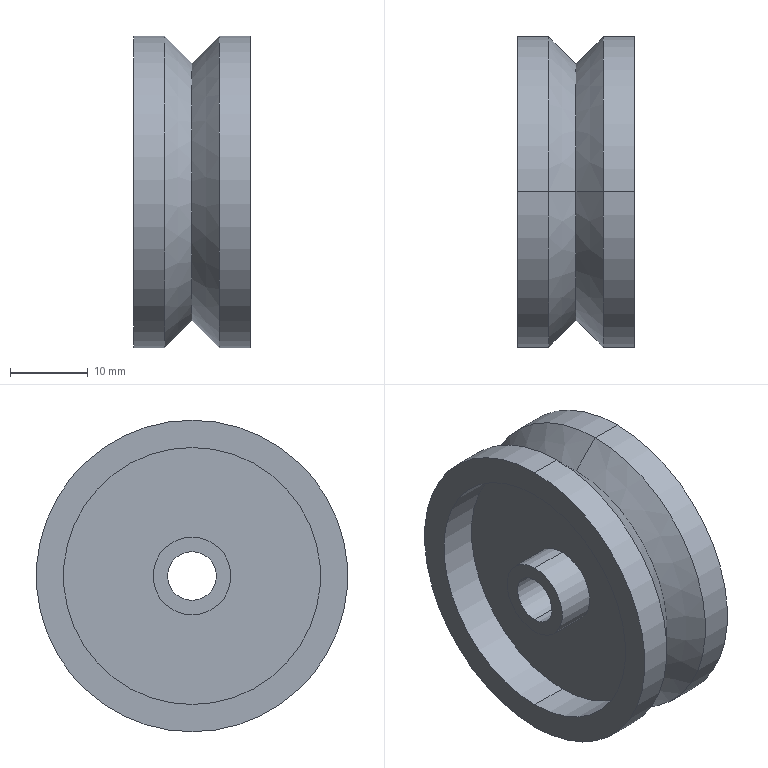Part | SolidWorks | features Revolution 1 | 1 solid | 24 faces | box 15 x 40 x 40 mm | volume 9172 mm3 | cylinder 14 | plane 6 | cone 4 | commonest cylinder face diameters 10 x4 33 x4 40 x4 6.25 x2
STEP:
#1=CARTESIAN_POINT('',(0.,0.,0.6496));
#2=VERTEX_POINT('',#1);
#3=CARTESIAN_POINT('',(0.,0.,-0.6496));
#4=VERTEX_POINT('',#3);
#5=CARTESIAN_POINT('',(0.,0.,0.));
#6=DIRECTION('',(-1.,0.,0.));
#7=DIRECTION('',(0.,0.,1.));
#8=AXIS2_PLACEMENT_3D('',#5,#6,#7);
#9=CIRCLE('',#8,0.6496);
#10=EDGE_CURVE('',#2,#4,#9,.T.);
#11=ORIENTED_EDGE('',*,*,#10,.F.);
#12=CARTESIAN_POINT('',(0.1378,0.,0.7874));
#13=VERTEX_POINT('',#12);
#14=CARTESIAN_POINT('',(0.1378,0.,0.7874));
#15=DIRECTION('',(0.7071,0.,0.7071));
#16=VECTOR('',#15,39.37);
#17=LINE('',#14,#16);
#18=EDGE_CURVE('',#2,#13,#17,.T.);
#19=ORIENTED_EDGE('',*,*,#18,.T.);
#20=CARTESIAN_POINT('',(0.1378,0.,-0.7874));
#21=VERTEX_POINT('',#20);
#22=CARTESIAN_POINT('',(0.1378,0.,0.));
#23=DIRECTION('',(-1.,0.,0.));
#24=DIRECTION('',(0.,0.,1.));
#25=AXIS2_PLACEMENT_3D('',#22,#23,#24);
#26=CIRCLE('',#25,0.7874);
#27=EDGE_CURVE('',#13,#21,#26,.T.);
#28=ORIENTED_EDGE('',*,*,#27,.T.);
#29=CARTESIAN_POINT('',(0.1378,0.,-0.7874));
#30=DIRECTION('',(0.7071,0.,-0.7071));
#31=VECTOR('',#30,39.37);
#32=LINE('',#29,#31);
#33=EDGE_CURVE('',#4,#21,#32,.T.);
#34=ORIENTED_EDGE('',*,*,#33,.F.);
#35=EDGE_LOOP('',(#11,#19,#28,#34));
#36=FACE_OUTER_BOUND('',#35,.T.);
#37=CARTESIAN_POINT('',(0.1378,0.,0.));
#38=DIRECTION('',(1.,0.,0.));
#39=DIRECTION('',(0.,0.,-1.));
#40=AXIS2_PLACEMENT_3D('',#37,#38,#39);
#41=CONICAL_SURFACE('',#40,0.7874,0.7854);
#42=ADVANCED_FACE('',(#36),#41,.T.);
#43=CARTESIAN_POINT('',(0.2953,0.,0.7874));
#44=VERTEX_POINT('',#43);
#45=CARTESIAN_POINT('',(0.2953,0.,-0.7874));
#46=VERTEX_POINT('',#45);
#47=CARTESIAN_POINT('',(0.2953,0.,0.));
#48=DIRECTION('',(-1.,0.,0.));
#49=DIRECTION('',(0.,0.,1.));
#50=AXIS2_PLACEMENT_3D('',#47,#48,#49);
#51=CIRCLE('',#50,0.7874);
#52=EDGE_CURVE('',#44,#46,#51,.T.);
#53=ORIENTED_EDGE('',*,*,#52,.T.);
#54=CARTESIAN_POINT('',(-1.791,0.,-0.7874));
#55=DIRECTION('',(-1.,0.,0.));
#56=VECTOR('',#55,39.37);
#57=LINE('',#54,#56);
#58=EDGE_CURVE('',#46,#21,#57,.T.);
#59=ORIENTED_EDGE('',*,*,#58,.T.);
#60=ORIENTED_EDGE('',*,*,#27,.F.);
#61=CARTESIAN_POINT('',(-1.791,0.,0.7874));
#62=DIRECTION('',(-1.,0.,0.));
#63=VECTOR('',#62,39.37);
#64=LINE('',#61,#63);
#65=EDGE_CURVE('',#44,#13,#64,.T.);
#66=ORIENTED_EDGE('',*,*,#65,.F.);
#67=EDGE_LOOP('',(#53,#59,#60,#66));
#68=FACE_OUTER_BOUND('',#67,.T.);
#69=CARTESIAN_POINT('',(-1.791,0.,0.));
#70=DIRECTION('',(-1.,0.,0.));
#71=DIRECTION('',(0.,0.,1.));
#72=AXIS2_PLACEMENT_3D('',#69,#70,#71);
#73=CYLINDRICAL_SURFACE('',#72,0.7874);
#74=ADVANCED_FACE('',(#68),#73,.T.);
#75=CARTESIAN_POINT('',(0.2953,0.,-0.6496));
#76=VERTEX_POINT('',#75);
#77=CARTESIAN_POINT('',(0.2953,0.,0.6496));
#78=VERTEX_POINT('',#77);
#79=CARTESIAN_POINT('',(0.2953,0.,0.));
#80=DIRECTION('',(-1.,0.,0.));
#81=DIRECTION('',(0.,0.,1.));
#82=AXIS2_PLACEMENT_3D('',#79,#80,#81);
#83=CIRCLE('',#82,0.6496);
#84=EDGE_CURVE('',#76,#78,#83,.T.);
#85=ORIENTED_EDGE('',*,*,#84,.F.);
#86=CARTESIAN_POINT('',(0.09843,0.,-0.6496));
#87=VERTEX_POINT('',#86);
#88=CARTESIAN_POINT('',(-1.791,0.,-0.6496));
#89=DIRECTION('',(-1.,0.,0.));
#90=VECTOR('',#89,39.37);
#91=LINE('',#88,#90);
#92=EDGE_CURVE('',#76,#87,#91,.T.);
#93=ORIENTED_EDGE('',*,*,#92,.T.);
#94=CARTESIAN_POINT('',(0.09843,0.,0.6496));
#95=VERTEX_POINT('',#94);
#96=CARTESIAN_POINT('',(0.09843,0.,0.));
#97=DIRECTION('',(-1.,0.,0.));
#98=DIRECTION('',(0.,0.,1.));
#99=AXIS2_PLACEMENT_3D('',#96,#97,#98);
#100=CIRCLE('',#99,0.6496);
#101=EDGE_CURVE('',#87,#95,#100,.T.);
#102=ORIENTED_EDGE('',*,*,#101,.T.);
#103=CARTESIAN_POINT('',(-1.791,0.,0.6496));
#104=DIRECTION('',(-1.,0.,0.));
#105=VECTOR('',#104,39.37);
#106=LINE('',#103,#105);
#107=EDGE_CURVE('',#78,#95,#106,.T.);
#108=ORIENTED_EDGE('',*,*,#107,.F.);
#109=EDGE_LOOP('',(#85,#93,#102,#108));
#110=FACE_OUTER_BOUND('',#109,.T.);
#111=CARTESIAN_POINT('',(-1.791,0.,0.));
#112=DIRECTION('',(-1.,0.,0.));
#113=DIRECTION('',(0.,0.,1.));
#114=AXIS2_PLACEMENT_3D('',#111,#112,#113);
#115=CYLINDRICAL_SURFACE('',#114,0.6496);
#116=ADVANCED_FACE('',(#110),#115,.F.);
#117=CARTESIAN_POINT('',(0.2953,0.,0.1969));
#118=VERTEX_POINT('',#117);
#119=CARTESIAN_POINT('',(0.2953,0.,-0.1969));
#120=VERTEX_POINT('',#119);
#121=CARTESIAN_POINT('',(0.2953,0.,0.));
#122=DIRECTION('',(-1.,0.,0.));
#123=DIRECTION('',(0.,0.,1.));
#124=AXIS2_PLACEMENT_3D('',#121,#122,#123);
#125=CIRCLE('',#124,0.1969);
#126=EDGE_CURVE('',#118,#120,#125,.T.);
#127=ORIENTED_EDGE('',*,*,#126,.T.);
#128=CARTESIAN_POINT('',(0.09843,0.,-0.1969));
#129=VERTEX_POINT('',#128);
#130=CARTESIAN_POINT('',(-1.791,0.,-0.1969));
#131=DIRECTION('',(-1.,0.,0.));
#132=VECTOR('',#131,39.37);
#133=LINE('',#130,#132);
#134=EDGE_CURVE('',#120,#129,#133,.T.);
#135=ORIENTED_EDGE('',*,*,#134,.T.);
#136=CARTESIAN_POINT('',(0.09843,0.,0.1969));
#137=VERTEX_POINT('',#136);
#138=CARTESIAN_POINT('',(0.09843,0.,0.));
#139=DIRECTION('',(-1.,0.,0.));
#140=DIRECTION('',(0.,0.,1.));
#141=AXIS2_PLACEMENT_3D('',#138,#139,#140);
#142=CIRCLE('',#141,0.1969);
#143=EDGE_CURVE('',#137,#129,#142,.T.);
#144=ORIENTED_EDGE('',*,*,#143,.F.);
#145=CARTESIAN_POINT('',(-1.791,0.,0.1969));
#146=DIRECTION('',(-1.,0.,0.));
#147=VECTOR('',#146,39.37);
#148=LINE('',#145,#147);
#149=EDGE_CURVE('',#118,#137,#148,.T.);
#150=ORIENTED_EDGE('',*,*,#149,.F.);
#151=EDGE_LOOP('',(#127,#135,#144,#150));
#152=FACE_OUTER_BOUND('',#151,.T.);
#153=CARTESIAN_POINT('',(-1.791,0.,0.));
#154=DIRECTION('',(-1.,0.,0.));
#155=DIRECTION('',(0.,0.,1.));
#156=AXIS2_PLACEMENT_3D('',#153,#154,#155);
#157=CYLINDRICAL_SURFACE('',#156,0.1969);
#158=ADVANCED_FACE('',(#152),#157,.T.);
#159=CARTESIAN_POINT('',(0.2953,0.,-0.123));
#160=VERTEX_POINT('',#159);
#161=CARTESIAN_POINT('',(0.2953,0.,0.123));
#162=VERTEX_POINT('',#161);
#163=CARTESIAN_POINT('',(0.2953,0.,0.));
#164=DIRECTION('',(-1.,0.,0.));
#165=DIRECTION('',(0.,0.,1.));
#166=AXIS2_PLACEMENT_3D('',#163,#164,#165);
#167=CIRCLE('',#166,0.123);
#168=EDGE_CURVE('',#160,#162,#167,.T.);
#169=ORIENTED_EDGE('',*,*,#168,.F.);
#170=CARTESIAN_POINT('',(-0.2953,0.,-0.123));
#171=VERTEX_POINT('',#170);
#172=CARTESIAN_POINT('',(-1.791,0.,-0.123));
#173=DIRECTION('',(-1.,0.,0.));
#174=VECTOR('',#173,39.37);
#175=LINE('',#172,#174);
#176=EDGE_CURVE('',#160,#171,#175,.T.);
#177=ORIENTED_EDGE('',*,*,#176,.T.);
#178=CARTESIAN_POINT('',(-0.2953,0.,0.123));
#179=VERTEX_POINT('',#178);
#180=CARTESIAN_POINT('',(-0.2953,0.,0.));
#181=DIRECTION('',(-1.,0.,0.));
#182=DIRECTION('',(0.,0.,1.));
#183=AXIS2_PLACEMENT_3D('',#180,#181,#182);
#184=CIRCLE('',#183,0.123);
#185=EDGE_CURVE('',#171,#179,#184,.T.);
#186=ORIENTED_EDGE('',*,*,#185,.T.);
#187=CARTESIAN_POINT('',(-1.791,0.,0.123));
#188=DIRECTION('',(-1.,0.,0.));
#189=VECTOR('',#188,39.37);
#190=LINE('',#187,#189);
#191=EDGE_CURVE('',#162,#179,#190,.T.);
#192=ORIENTED_EDGE('',*,*,#191,.F.);
#193=EDGE_LOOP('',(#169,#177,#186,#192));
#194=FACE_OUTER_BOUND('',#193,.T.);
#195=CARTESIAN_POINT('',(-1.791,0.,0.));
#196=DIRECTION('',(-1.,0.,0.));
#197=DIRECTION('',(0.,0.,1.));
#198=AXIS2_PLACEMENT_3D('',#195,#196,#197);
#199=CYLINDRICAL_SURFACE('',#198,0.123);
#200=ADVANCED_FACE('',(#194),#199,.F.);
#201=CARTESIAN_POINT('',(-0.09843,0.,0.1969));
#202=VERTEX_POINT('',#201);
#203=CARTESIAN_POINT('',(-0.09843,0.,-0.1969));
#204=VERTEX_POINT('',#203);
#205=CARTESIAN_POINT('',(-0.09843,0.,0.));
#206=DIRECTION('',(-1.,0.,0.));
#207=DIRECTION('',(0.,0.,1.));
#208=AXIS2_PLACEMENT_3D('',#205,#206,#207);
#209=CIRCLE('',#208,0.1969);
#210=EDGE_CURVE('',#202,#204,#209,.T.);
#211=ORIENTED_EDGE('',*,*,#210,.T.);
#212=CARTESIAN_POINT('',(-0.2953,0.,-0.1969));
#213=VERTEX_POINT('',#212);
#214=CARTESIAN_POINT('',(-1.791,0.,-0.1969));
#215=DIRECTION('',(-1.,0.,0.));
#216=VECTOR('',#215,39.37);
#217=LINE('',#214,#216);
#218=EDGE_CURVE('',#204,#213,#217,.T.);
#219=ORIENTED_EDGE('',*,*,#218,.T.);
#220=CARTESIAN_POINT('',(-0.2953,0.,0.1969));
#221=VERTEX_POINT('',#220);
#222=CARTESIAN_POINT('',(-0.2953,0.,0.));
#223=DIRECTION('',(-1.,0.,0.));
#224=DIRECTION('',(0.,0.,1.));
#225=AXIS2_PLACEMENT_3D('',#222,#223,#224);
#226=CIRCLE('',#225,0.1969);
#227=EDGE_CURVE('',#221,#213,#226,.T.);
#228=ORIENTED_EDGE('',*,*,#227,.F.);
#229=CARTESIAN_POINT('',(-1.791,0.,0.1969));
#230=DIRECTION('',(-1.,0.,0.));
#231=VECTOR('',#230,39.37);
#232=LINE('',#229,#231);
#233=EDGE_CURVE('',#202,#221,#232,.T.);
#234=ORIENTED_EDGE('',*,*,#233,.F.);
#235=EDGE_LOOP('',(#211,#219,#228,#234));
#236=FACE_OUTER_BOUND('',#235,.T.);
#237=CARTESIAN_POINT('',(-1.791,0.,0.));
#238=DIRECTION('',(-1.,0.,0.));
#239=DIRECTION('',(0.,0.,1.));
#240=AXIS2_PLACEMENT_3D('',#237,#238,#239);
#241=CYLINDRICAL_SURFACE('',#240,0.1969);
#242=ADVANCED_FACE('',(#236),#241,.T.);
#243=CARTESIAN_POINT('',(-0.09843,0.,-0.6496));
#244=VERTEX_POINT('',#243);
#245=CARTESIAN_POINT('',(-0.09843,0.,0.6496));
#246=VERTEX_POINT('',#245);
#247=CARTESIAN_POINT('',(-0.09843,0.,0.));
#248=DIRECTION('',(-1.,0.,0.));
#249=DIRECTION('',(0.,0.,1.));
#250=AXIS2_PLACEMENT_3D('',#247,#248,#249);
#251=CIRCLE('',#250,0.6496);
#252=EDGE_CURVE('',#244,#246,#251,.T.);
#253=ORIENTED_EDGE('',*,*,#252,.F.);
#254=CARTESIAN_POINT('',(-0.2953,0.,-0.6496));
#255=VERTEX_POINT('',#254);
#256=CARTESIAN_POINT('',(-1.791,0.,-0.6496));
#257=DIRECTION('',(-1.,0.,0.));
#258=VECTOR('',#257,39.37);
#259=LINE('',#256,#258);
#260=EDGE_CURVE('',#244,#255,#259,.T.);
#261=ORIENTED_EDGE('',*,*,#260,.T.);
#262=CARTESIAN_POINT('',(-0.2953,0.,0.6496));
#263=VERTEX_POINT('',#262);
#264=CARTESIAN_POINT('',(-0.2953,0.,0.));
#265=DIRECTION('',(-1.,0.,0.));
#266=DIRECTION('',(0.,0.,1.));
#267=AXIS2_PLACEMENT_3D('',#264,#265,#266);
#268=CIRCLE('',#267,0.6496);
#269=EDGE_CURVE('',#255,#263,#268,.T.);
#270=ORIENTED_EDGE('',*,*,#269,.T.);
#271=CARTESIAN_POINT('',(-1.791,0.,0.6496));
#272=DIRECTION('',(-1.,0.,0.));
#273=VECTOR('',#272,39.37);
#274=LINE('',#271,#273);
#275=EDGE_CURVE('',#246,#263,#274,.T.);
#276=ORIENTED_EDGE('',*,*,#275,.F.);
#277=EDGE_LOOP('',(#253,#261,#270,#276));
#278=FACE_OUTER_BOUND('',#277,.T.);
#279=CARTESIAN_POINT('',(-1.791,0.,0.));
#280=DIRECTION('',(-1.,0.,0.));
#281=DIRECTION('',(0.,0.,1.));
#282=AXIS2_PLACEMENT_3D('',#279,#280,#281);
#283=CYLINDRICAL_SURFACE('',#282,0.6496);
#284=ADVANCED_FACE('',(#278),#283,.F.);
#285=CARTESIAN_POINT('',(-0.1378,0.,0.7874));
#286=VERTEX_POINT('',#285);
#287=CARTESIAN_POINT('',(-0.1378,0.,-0.7874));
#288=VERTEX_POINT('',#287);
#289=CARTESIAN_POINT('',(-0.1378,0.,0.));
#290=DIRECTION('',(-1.,0.,0.));
#291=DIRECTION('',(0.,0.,1.));
#292=AXIS2_PLACEMENT_3D('',#289,#290,#291);
#293=CIRCLE('',#292,0.7874);
#294=EDGE_CURVE('',#286,#288,#293,.T.);
#295=ORIENTED_EDGE('',*,*,#294,.T.);
#296=CARTESIAN_POINT('',(-0.2953,0.,-0.7874));
#297=VERTEX_POINT('',#296);
#298=CARTESIAN_POINT('',(-1.791,0.,-0.7874));
#299=DIRECTION('',(-1.,0.,0.));
#300=VECTOR('',#299,39.37);
#301=LINE('',#298,#300);
#302=EDGE_CURVE('',#288,#297,#301,.T.);
#303=ORIENTED_EDGE('',*,*,#302,.T.);
#304=CARTESIAN_POINT('',(-0.2953,0.,0.7874));
#305=VERTEX_POINT('',#304);
#306=CARTESIAN_POINT('',(-0.2953,0.,0.));
#307=DIRECTION('',(-1.,0.,0.));
#308=DIRECTION('',(0.,0.,1.));
#309=AXIS2_PLACEMENT_3D('',#306,#307,#308);
#310=CIRCLE('',#309,0.7874);
#311=EDGE_CURVE('',#305,#297,#310,.T.);
#312=ORIENTED_EDGE('',*,*,#311,.F.);
#313=CARTESIAN_POINT('',(-1.791,0.,0.7874));
#314=DIRECTION('',(-1.,0.,0.));
#315=VECTOR('',#314,39.37);
#316=LINE('',#313,#315);
#317=EDGE_CURVE('',#286,#305,#316,.T.);
#318=ORIENTED_EDGE('',*,*,#317,.F.);
#319=EDGE_LOOP('',(#295,#303,#312,#318));
#320=FACE_OUTER_BOUND('',#319,.T.);
#321=CARTESIAN_POINT('',(-1.791,0.,0.));
#322=DIRECTION('',(-1.,0.,0.));
#323=DIRECTION('',(0.,0.,1.));
#324=AXIS2_PLACEMENT_3D('',#321,#322,#323);
#325=CYLINDRICAL_SURFACE('',#324,0.7874);
#326=ADVANCED_FACE('',(#320),#325,.T.);
#327=ORIENTED_EDGE('',*,*,#10,.T.);
#328=CARTESIAN_POINT('',(0.,0.,-0.6496));
#329=DIRECTION('',(-0.7071,0.,-0.7071));
#330=VECTOR('',#329,39.37);
#331=LINE('',#328,#330);
#332=EDGE_CURVE('',#4,#288,#331,.T.);
#333=ORIENTED_EDGE('',*,*,#332,.T.);
#334=ORIENTED_EDGE('',*,*,#294,.F.);
#335=CARTESIAN_POINT('',(0.,0.,0.6496));
#336=DIRECTION('',(-0.7071,0.,0.7071));
#337=VECTOR('',#336,39.37);
#338=LINE('',#335,#337);
#339=EDGE_CURVE('',#2,#286,#338,.T.);
#340=ORIENTED_EDGE('',*,*,#339,.F.);
#341=EDGE_LOOP('',(#327,#333,#334,#340));
#342=FACE_OUTER_BOUND('',#341,.T.);
#343=CARTESIAN_POINT('',(0.,0.,0.));
#344=DIRECTION('',(-1.,0.,0.));
#345=DIRECTION('',(0.,0.,1.));
#346=AXIS2_PLACEMENT_3D('',#343,#344,#345);
#347=CONICAL_SURFACE('',#346,0.6496,0.7854);
#348=ADVANCED_FACE('',(#342),#347,.T.);
#349=ORIENTED_EDGE('',*,*,#332,.F.);
#350=CARTESIAN_POINT('',(0.,0.,0.));
#351=DIRECTION('',(-1.,0.,0.));
#352=DIRECTION('',(0.,0.,1.));
#353=AXIS2_PLACEMENT_3D('',#350,#351,#352);
#354=CIRCLE('',#353,0.6496);
#355=EDGE_CURVE('',#4,#2,#354,.T.);
#356=ORIENTED_EDGE('',*,*,#355,.T.);
#357=ORIENTED_EDGE('',*,*,#339,.T.);
#358=CARTESIAN_POINT('',(-0.1378,0.,0.));
#359=DIRECTION('',(-1.,0.,0.));
#360=DIRECTION('',(0.,0.,1.));
#361=AXIS2_PLACEMENT_3D('',#358,#359,#360);
#362=CIRCLE('',#361,0.7874);
#363=EDGE_CURVE('',#288,#286,#362,.T.);
#364=ORIENTED_EDGE('',*,*,#363,.F.);
#365=EDGE_LOOP('',(#349,#356,#357,#364));
#366=FACE_OUTER_BOUND('',#365,.T.);
#367=CARTESIAN_POINT('',(0.,0.,0.));
#368=DIRECTION('',(-1.,0.,0.));
#369=DIRECTION('',(0.,0.,1.));
#370=AXIS2_PLACEMENT_3D('',#367,#368,#369);
#371=CONICAL_SURFACE('',#370,0.6496,0.7854);
#372=ADVANCED_FACE('',(#366),#371,.T.);
#373=ORIENTED_EDGE('',*,*,#302,.F.);
#374=ORIENTED_EDGE('',*,*,#363,.T.);
#375=ORIENTED_EDGE('',*,*,#317,.T.);
#376=CARTESIAN_POINT('',(-0.2953,0.,0.));
#377=DIRECTION('',(-1.,0.,0.));
#378=DIRECTION('',(0.,0.,1.));
#379=AXIS2_PLACEMENT_3D('',#376,#377,#378);
#380=CIRCLE('',#379,0.7874);
#381=EDGE_CURVE('',#297,#305,#380,.T.);
#382=ORIENTED_EDGE('',*,*,#381,.F.);
#383=EDGE_LOOP('',(#373,#374,#375,#382));
#384=FACE_OUTER_BOUND('',#383,.T.);
#385=CARTESIAN_POINT('',(-1.791,0.,0.));
#386=DIRECTION('',(-1.,0.,0.));
#387=DIRECTION('',(0.,0.,1.));
#388=AXIS2_PLACEMENT_3D('',#385,#386,#387);
#389=CYLINDRICAL_SURFACE('',#388,0.7874);
#390=ADVANCED_FACE('',(#384),#389,.T.);
#391=CARTESIAN_POINT('',(-0.2953,0.,0.));
#392=DIRECTION('',(-1.,0.,0.));
#393=DIRECTION('',(0.,0.,1.));
#394=AXIS2_PLACEMENT_3D('',#391,#392,#393);
#395=CIRCLE('',#394,0.6496);
#396=EDGE_CURVE('',#263,#255,#395,.T.);
#397=ORIENTED_EDGE('',*,*,#396,.F.);
#398=ORIENTED_EDGE('',*,*,#269,.F.);
#399=EDGE_LOOP('',(#397,#398));
#400=FACE_BOUND('',#399,.T.);
#401=ORIENTED_EDGE('',*,*,#311,.T.);
#402=ORIENTED_EDGE('',*,*,#381,.T.);
#403=EDGE_LOOP('',(#401,#402));
#404=FACE_OUTER_BOUND('',#403,.T.);
#405=CARTESIAN_POINT('',(-0.2953,0.7874,0.));
#406=DIRECTION('',(1.,0.,0.));
#407=DIRECTION('',(0.,0.,-1.));
#408=AXIS2_PLACEMENT_3D('',#405,#406,#407);
#409=PLANE('',#408);
#410=ADVANCED_FACE('',(#400,#404),#409,.F.);
#411=ORIENTED_EDGE('',*,*,#260,.F.);
#412=CARTESIAN_POINT('',(-0.09843,0.,0.));
#413=DIRECTION('',(-1.,0.,0.));
#414=DIRECTION('',(0.,0.,1.));
#415=AXIS2_PLACEMENT_3D('',#412,#413,#414);
#416=CIRCLE('',#415,0.6496);
#417=EDGE_CURVE('',#246,#244,#416,.T.);
#418=ORIENTED_EDGE('',*,*,#417,.F.);
#419=ORIENTED_EDGE('',*,*,#275,.T.);
#420=ORIENTED_EDGE('',*,*,#396,.T.);
#421=EDGE_LOOP('',(#411,#418,#419,#420));
#422=FACE_OUTER_BOUND('',#421,.T.);
#423=CARTESIAN_POINT('',(-1.791,0.,0.));
#424=DIRECTION('',(-1.,0.,0.));
#425=DIRECTION('',(0.,0.,1.));
#426=AXIS2_PLACEMENT_3D('',#423,#424,#425);
#427=CYLINDRICAL_SURFACE('',#426,0.6496);
#428=ADVANCED_FACE('',(#422),#427,.F.);
#429=ORIENTED_EDGE('',*,*,#210,.F.);
#430=CARTESIAN_POINT('',(-0.09843,0.,0.));
#431=DIRECTION('',(-1.,0.,0.));
#432=DIRECTION('',(0.,0.,1.));
#433=AXIS2_PLACEMENT_3D('',#430,#431,#432);
#434=CIRCLE('',#433,0.1969);
#435=EDGE_CURVE('',#204,#202,#434,.T.);
#436=ORIENTED_EDGE('',*,*,#435,.F.);
#437=EDGE_LOOP('',(#429,#436));
#438=FACE_BOUND('',#437,.T.);
#439=ORIENTED_EDGE('',*,*,#417,.T.);
#440=ORIENTED_EDGE('',*,*,#252,.T.);
#441=EDGE_LOOP('',(#439,#440));
#442=FACE_OUTER_BOUND('',#441,.T.);
#443=CARTESIAN_POINT('',(-0.09843,0.6496,0.));
#444=DIRECTION('',(1.,0.,0.));
#445=DIRECTION('',(0.,0.,-1.));
#446=AXIS2_PLACEMENT_3D('',#443,#444,#445);
#447=PLANE('',#446);
#448=ADVANCED_FACE('',(#438,#442),#447,.F.);
#449=ORIENTED_EDGE('',*,*,#218,.F.);
#450=ORIENTED_EDGE('',*,*,#435,.T.);
#451=ORIENTED_EDGE('',*,*,#233,.T.);
#452=CARTESIAN_POINT('',(-0.2953,0.,0.));
#453=DIRECTION('',(-1.,0.,0.));
#454=DIRECTION('',(0.,0.,1.));
#455=AXIS2_PLACEMENT_3D('',#452,#453,#454);
#456=CIRCLE('',#455,0.1969);
#457=EDGE_CURVE('',#213,#221,#456,.T.);
#458=ORIENTED_EDGE('',*,*,#457,.F.);
#459=EDGE_LOOP('',(#449,#450,#451,#458));
#460=FACE_OUTER_BOUND('',#459,.T.);
#461=CARTESIAN_POINT('',(-1.791,0.,0.));
#462=DIRECTION('',(-1.,0.,0.));
#463=DIRECTION('',(0.,0.,1.));
#464=AXIS2_PLACEMENT_3D('',#461,#462,#463);
#465=CYLINDRICAL_SURFACE('',#464,0.1969);
#466=ADVANCED_FACE('',(#460),#465,.T.);
#467=CARTESIAN_POINT('',(-0.2953,0.,0.));
#468=DIRECTION('',(-1.,0.,0.));
#469=DIRECTION('',(0.,0.,1.));
#470=AXIS2_PLACEMENT_3D('',#467,#468,#469);
#471=CIRCLE('',#470,0.123);
#472=EDGE_CURVE('',#179,#171,#471,.T.);
#473=ORIENTED_EDGE('',*,*,#472,.F.);
#474=ORIENTED_EDGE('',*,*,#185,.F.);
#475=EDGE_LOOP('',(#473,#474));
#476=FACE_BOUND('',#475,.T.);
#477=ORIENTED_EDGE('',*,*,#227,.T.);
#478=ORIENTED_EDGE('',*,*,#457,.T.);
#479=EDGE_LOOP('',(#477,#478));
#480=FACE_OUTER_BOUND('',#479,.T.);
#481=CARTESIAN_POINT('',(-0.2953,0.1969,0.));
#482=DIRECTION('',(1.,0.,0.));
#483=DIRECTION('',(0.,0.,-1.));
#484=AXIS2_PLACEMENT_3D('',#481,#482,#483);
#485=PLANE('',#484);
#486=ADVANCED_FACE('',(#476,#480),#485,.F.);
#487=ORIENTED_EDGE('',*,*,#176,.F.);
#488=CARTESIAN_POINT('',(0.2953,0.,0.));
#489=DIRECTION('',(-1.,0.,0.));
#490=DIRECTION('',(0.,0.,1.));
#491=AXIS2_PLACEMENT_3D('',#488,#489,#490);
#492=CIRCLE('',#491,0.123);
#493=EDGE_CURVE('',#162,#160,#492,.T.);
#494=ORIENTED_EDGE('',*,*,#493,.F.);
#495=ORIENTED_EDGE('',*,*,#191,.T.);
#496=ORIENTED_EDGE('',*,*,#472,.T.);
#497=EDGE_LOOP('',(#487,#494,#495,#496));
#498=FACE_OUTER_BOUND('',#497,.T.);
#499=CARTESIAN_POINT('',(-1.791,0.,0.));
#500=DIRECTION('',(-1.,0.,0.));
#501=DIRECTION('',(0.,0.,1.));
#502=AXIS2_PLACEMENT_3D('',#499,#500,#501);
#503=CYLINDRICAL_SURFACE('',#502,0.123);
#504=ADVANCED_FACE('',(#498),#503,.F.);
#505=ORIENTED_EDGE('',*,*,#126,.F.);
#506=CARTESIAN_POINT('',(0.2953,0.,0.));
#507=DIRECTION('',(-1.,0.,0.));
#508=DIRECTION('',(0.,0.,1.));
#509=AXIS2_PLACEMENT_3D('',#506,#507,#508);
#510=CIRCLE('',#509,0.1969);
#511=EDGE_CURVE('',#120,#118,#510,.T.);
#512=ORIENTED_EDGE('',*,*,#511,.F.);
#513=EDGE_LOOP('',(#505,#512));
#514=FACE_OUTER_BOUND('',#513,.T.);
#515=ORIENTED_EDGE('',*,*,#493,.T.);
#516=ORIENTED_EDGE('',*,*,#168,.T.);
#517=EDGE_LOOP('',(#515,#516));
#518=FACE_BOUND('',#517,.T.);
#519=CARTESIAN_POINT('',(0.2953,0.123,0.));
#520=DIRECTION('',(-1.,0.,0.));
#521=DIRECTION('',(0.,0.,1.));
#522=AXIS2_PLACEMENT_3D('',#519,#520,#521);
#523=PLANE('',#522);
#524=ADVANCED_FACE('',(#514,#518),#523,.F.);
#525=ORIENTED_EDGE('',*,*,#134,.F.);
#526=ORIENTED_EDGE('',*,*,#511,.T.);
#527=ORIENTED_EDGE('',*,*,#149,.T.);
#528=CARTESIAN_POINT('',(0.09843,0.,0.));
#529=DIRECTION('',(-1.,0.,0.));
#530=DIRECTION('',(0.,0.,1.));
#531=AXIS2_PLACEMENT_3D('',#528,#529,#530);
#532=CIRCLE('',#531,0.1969);
#533=EDGE_CURVE('',#129,#137,#532,.T.);
#534=ORIENTED_EDGE('',*,*,#533,.F.);
#535=EDGE_LOOP('',(#525,#526,#527,#534));
#536=FACE_OUTER_BOUND('',#535,.T.);
#537=CARTESIAN_POINT('',(-1.791,0.,0.));
#538=DIRECTION('',(-1.,0.,0.));
#539=DIRECTION('',(0.,0.,1.));
#540=AXIS2_PLACEMENT_3D('',#537,#538,#539);
#541=CYLINDRICAL_SURFACE('',#540,0.1969);
#542=ADVANCED_FACE('',(#536),#541,.T.);
#543=CARTESIAN_POINT('',(0.09843,0.,0.));
#544=DIRECTION('',(-1.,0.,0.));
#545=DIRECTION('',(0.,0.,1.));
#546=AXIS2_PLACEMENT_3D('',#543,#544,#545);
#547=CIRCLE('',#546,0.6496);
#548=EDGE_CURVE('',#95,#87,#547,.T.);
#549=ORIENTED_EDGE('',*,*,#548,.F.);
#550=ORIENTED_EDGE('',*,*,#101,.F.);
#551=EDGE_LOOP('',(#549,#550));
#552=FACE_OUTER_BOUND('',#551,.T.);
#553=ORIENTED_EDGE('',*,*,#143,.T.);
#554=ORIENTED_EDGE('',*,*,#533,.T.);
#555=EDGE_LOOP('',(#553,#554));
#556=FACE_BOUND('',#555,.T.);
#557=CARTESIAN_POINT('',(0.09843,0.1969,0.));
#558=DIRECTION('',(-1.,0.,0.));
#559=DIRECTION('',(0.,0.,1.));
#560=AXIS2_PLACEMENT_3D('',#557,#558,#559);
#561=PLANE('',#560);
#562=ADVANCED_FACE('',(#552,#556),#561,.F.);
#563=ORIENTED_EDGE('',*,*,#92,.F.);
#564=CARTESIAN_POINT('',(0.2953,0.,0.));
#565=DIRECTION('',(-1.,0.,0.));
#566=DIRECTION('',(0.,0.,1.));
#567=AXIS2_PLACEMENT_3D('',#564,#565,#566);
#568=CIRCLE('',#567,0.6496);
#569=EDGE_CURVE('',#78,#76,#568,.T.);
#570=ORIENTED_EDGE('',*,*,#569,.F.);
#571=ORIENTED_EDGE('',*,*,#107,.T.);
#572=ORIENTED_EDGE('',*,*,#548,.T.);
#573=EDGE_LOOP('',(#563,#570,#571,#572));
#574=FACE_OUTER_BOUND('',#573,.T.);
#575=CARTESIAN_POINT('',(-1.791,0.,0.));
#576=DIRECTION('',(-1.,0.,0.));
#577=DIRECTION('',(0.,0.,1.));
#578=AXIS2_PLACEMENT_3D('',#575,#576,#577);
#579=CYLINDRICAL_SURFACE('',#578,0.6496);
#580=ADVANCED_FACE('',(#574),#579,.F.);
#581=ORIENTED_EDGE('',*,*,#52,.F.);
#582=CARTESIAN_POINT('',(0.2953,0.,0.));
#583=DIRECTION('',(-1.,0.,0.));
#584=DIRECTION('',(0.,0.,1.));
#585=AXIS2_PLACEMENT_3D('',#582,#583,#584);
#586=CIRCLE('',#585,0.7874);
#587=EDGE_CURVE('',#46,#44,#586,.T.);
#588=ORIENTED_EDGE('',*,*,#587,.F.);
#589=EDGE_LOOP('',(#581,#588));
#590=FACE_OUTER_BOUND('',#589,.T.);
#591=ORIENTED_EDGE('',*,*,#569,.T.);
#592=ORIENTED_EDGE('',*,*,#84,.T.);
#593=EDGE_LOOP('',(#591,#592));
#594=FACE_BOUND('',#593,.T.);
#595=CARTESIAN_POINT('',(0.2953,0.6496,0.));
#596=DIRECTION('',(-1.,0.,0.));
#597=DIRECTION('',(0.,0.,1.));
#598=AXIS2_PLACEMENT_3D('',#595,#596,#597);
#599=PLANE('',#598);
#600=ADVANCED_FACE('',(#590,#594),#599,.F.);
#601=ORIENTED_EDGE('',*,*,#58,.F.);
#602=ORIENTED_EDGE('',*,*,#587,.T.);
#603=ORIENTED_EDGE('',*,*,#65,.T.);
#604=CARTESIAN_POINT('',(0.1378,0.,0.));
#605=DIRECTION('',(-1.,0.,0.));
#606=DIRECTION('',(0.,0.,1.));
#607=AXIS2_PLACEMENT_3D('',#604,#605,#606);
#608=CIRCLE('',#607,0.7874);
#609=EDGE_CURVE('',#21,#13,#608,.T.);
#610=ORIENTED_EDGE('',*,*,#609,.F.);
#611=EDGE_LOOP('',(#601,#602,#603,#610));
#612=FACE_OUTER_BOUND('',#611,.T.);
#613=CARTESIAN_POINT('',(-1.791,0.,0.));
#614=DIRECTION('',(-1.,0.,0.));
#615=DIRECTION('',(0.,0.,1.));
#616=AXIS2_PLACEMENT_3D('',#613,#614,#615);
#617=CYLINDRICAL_SURFACE('',#616,0.7874);
#618=ADVANCED_FACE('',(#612),#617,.T.);
#619=ORIENTED_EDGE('',*,*,#18,.F.);
#620=ORIENTED_EDGE('',*,*,#355,.F.);
#621=ORIENTED_EDGE('',*,*,#33,.T.);
#622=ORIENTED_EDGE('',*,*,#609,.T.);
#623=EDGE_LOOP('',(#619,#620,#621,#622));
#624=FACE_OUTER_BOUND('',#623,.T.);
#625=CARTESIAN_POINT('',(0.1378,0.,0.));
#626=DIRECTION('',(1.,0.,0.));
#627=DIRECTION('',(0.,0.,-1.));
#628=AXIS2_PLACEMENT_3D('',#625,#626,#627);
#629=CONICAL_SURFACE('',#628,0.7874,0.7854);
#630=ADVANCED_FACE('',(#624),#629,.T.);
#631=CLOSED_SHELL('',(#42,#74,#116,#158,#200,#242,#284,#326,#348,#372,#390,#410,#428,#448,#466,#486,#504,#524,#542,#562,#580,#600,#618,#630));
#632=MANIFOLD_SOLID_BREP('',#631);
#633=CARTESIAN_POINT('',(0.,0.,0.));
#634=DIRECTION('',(0.,0.,1.));
#635=DIRECTION('',(1.,0.,0.));
#636=AXIS2_PLACEMENT_3D('',#633,#634,#635);
#637=(LENGTH_UNIT()NAMED_UNIT(*)SI_UNIT($,.METRE.));
#638=LENGTH_MEASURE_WITH_UNIT(LENGTH_MEASURE(0.0254),#637);
#639=DIMENSIONAL_EXPONENTS(1.,0.,0.,0.,0.,0.,0.);
#640=(CONVERSION_BASED_UNIT('INCH',#638)LENGTH_UNIT()NAMED_UNIT(#639));
#641=UNCERTAINTY_MEASURE_WITH_UNIT(LENGTH_MEASURE(0.00001),#640,'','');
#642=(NAMED_UNIT(*)PLANE_ANGLE_UNIT()SI_UNIT($,.RADIAN.));
#643=(NAMED_UNIT(*)SI_UNIT($,.STERADIAN.)SOLID_ANGLE_UNIT());
#644=(GEOMETRIC_REPRESENTATION_CONTEXT(3)GLOBAL_UNCERTAINTY_ASSIGNED_CONTEXT((#641))GLOBAL_UNIT_ASSIGNED_CONTEXT((#640,#642,#643))REPRESENTATION_CONTEXT('',''));
#645=ADVANCED_BREP_SHAPE_REPRESENTATION('',(#632,#636),#644);